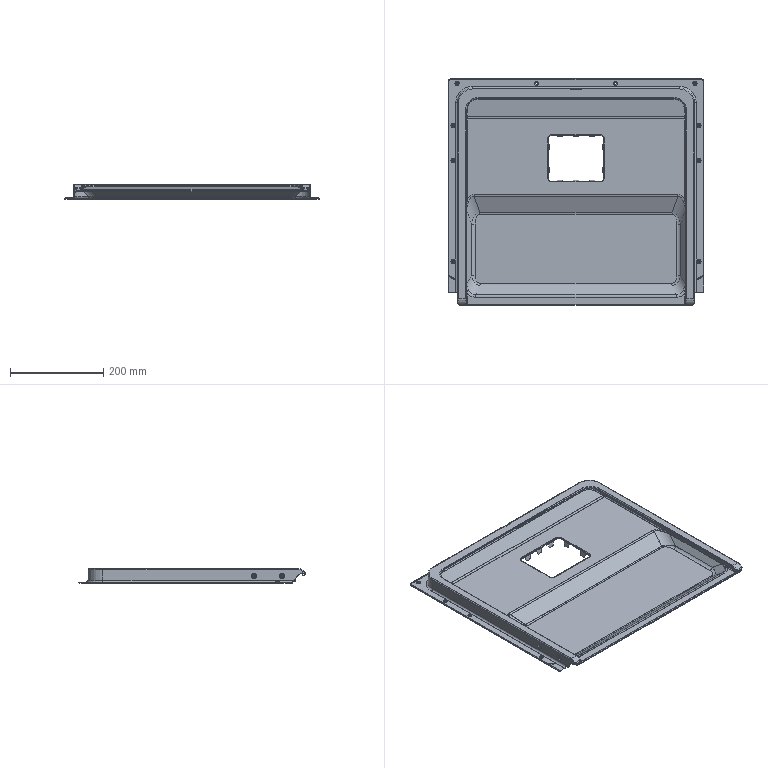Part | STEP file | ZXW722-L-30 | 1 solid | 796 faces | box 547 x 485.1 x 31.6 mm | volume 126508 mm3 | cylinder 255 | plane 195 | spline 166 | torus 122 | cone 28 | other 28 | sphere 2 | commonest cylinder face diameters 4 x46 4.2 x22 6 x22 1.6 x15 4.8 x14 3.2 x10